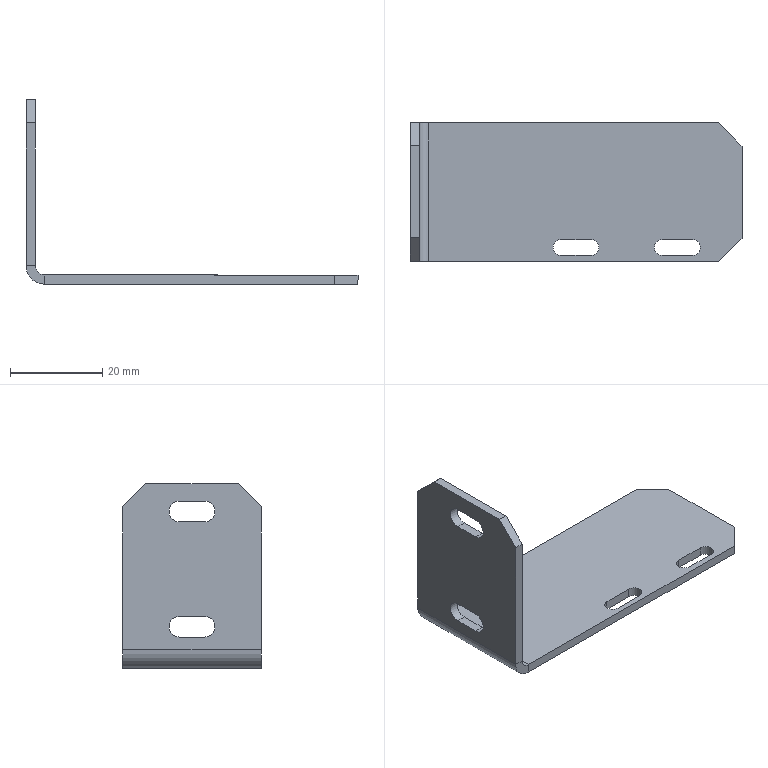Part | SolidWorks | features HoleWzd 2, Chamfer 1, EdgeFlange 1, FlatPattern 1, SMBaseFlange 1, SheetMetal 1 | 1 solid | 34 faces | box 72 x 30 x 40 mm | volume 6134 mm3 | plane 24 | cylinder 10 | commonest cylinder face diameters 3.4 x4 4.5 x4 4 x1 8 x1
STEP:
#1=CARTESIAN_POINT('',(37.3,-10.3,-20.));
#2=VERTEX_POINT('',#1);
#3=CARTESIAN_POINT('',(37.3,-13.7,-20.));
#4=VERTEX_POINT('',#3);
#5=CARTESIAN_POINT('',(37.3,-12.,-20.));
#6=DIRECTION('',(0.,0.,-1.));
#7=DIRECTION('',(0.,1.,0.));
#8=AXIS2_PLACEMENT_3D('',#5,#6,#7);
#9=CIRCLE('',#8,1.7);
#10=EDGE_CURVE('',#2,#4,#9,.T.);
#11=ORIENTED_EDGE('',*,*,#10,.F.);
#12=CARTESIAN_POINT('',(30.7,-10.3,-20.));
#13=VERTEX_POINT('',#12);
#14=CARTESIAN_POINT('',(37.3,-10.3,-20.));
#15=DIRECTION('',(-1.,0.,0.));
#16=VECTOR('',#15,1000.);
#17=LINE('',#14,#16);
#18=EDGE_CURVE('',#2,#13,#17,.T.);
#19=ORIENTED_EDGE('',*,*,#18,.T.);
#20=CARTESIAN_POINT('',(30.7,-13.7,-20.));
#21=VERTEX_POINT('',#20);
#22=CARTESIAN_POINT('',(30.7,-12.,-20.));
#23=DIRECTION('',(0.,0.,-1.));
#24=DIRECTION('',(0.,1.,0.));
#25=AXIS2_PLACEMENT_3D('',#22,#23,#24);
#26=CIRCLE('',#25,1.7);
#27=EDGE_CURVE('',#21,#13,#26,.T.);
#28=ORIENTED_EDGE('',*,*,#27,.F.);
#29=CARTESIAN_POINT('',(37.3,-13.7,-20.));
#30=DIRECTION('',(-1.,0.,0.));
#31=VECTOR('',#30,1000.);
#32=LINE('',#29,#31);
#33=EDGE_CURVE('',#4,#21,#32,.T.);
#34=ORIENTED_EDGE('',*,*,#33,.F.);
#35=EDGE_LOOP('',(#11,#19,#28,#34));
#36=FACE_BOUND('',#35,.T.);
#37=CARTESIAN_POINT('',(70.,10.,-20.));
#38=VERTEX_POINT('',#37);
#39=CARTESIAN_POINT('',(70.,-10.,-20.));
#40=VERTEX_POINT('',#39);
#41=CARTESIAN_POINT('',(70.,0.,-20.));
#42=DIRECTION('',(0.,-1.,0.));
#43=VECTOR('',#42,1000.);
#44=LINE('',#41,#43);
#45=EDGE_CURVE('',#38,#40,#44,.T.);
#46=ORIENTED_EDGE('',*,*,#45,.T.);
#47=CARTESIAN_POINT('',(65.,-15.,-20.));
#48=VERTEX_POINT('',#47);
#49=CARTESIAN_POINT('',(65.,-15.,-20.));
#50=DIRECTION('',(-0.7071,-0.7071,0.));
#51=VECTOR('',#50,1000.);
#52=LINE('',#49,#51);
#53=EDGE_CURVE('',#40,#48,#52,.T.);
#54=ORIENTED_EDGE('',*,*,#53,.T.);
#55=CARTESIAN_POINT('',(2.,-15.,-20.));
#56=VERTEX_POINT('',#55);
#57=CARTESIAN_POINT('',(0.,-15.,-20.));
#58=DIRECTION('',(-1.,0.,0.));
#59=VECTOR('',#58,1000.);
#60=LINE('',#57,#59);
#61=EDGE_CURVE('',#48,#56,#60,.T.);
#62=ORIENTED_EDGE('',*,*,#61,.T.);
#63=CARTESIAN_POINT('',(2.,15.,-20.));
#64=VERTEX_POINT('',#63);
#65=CARTESIAN_POINT('',(2.,-15.,-20.));
#66=DIRECTION('',(0.,-1.,0.));
#67=VECTOR('',#66,1000.);
#68=LINE('',#65,#67);
#69=EDGE_CURVE('',#64,#56,#68,.T.);
#70=ORIENTED_EDGE('',*,*,#69,.F.);
#71=CARTESIAN_POINT('',(65.,15.,-20.));
#72=VERTEX_POINT('',#71);
#73=CARTESIAN_POINT('',(0.,15.,-20.));
#74=DIRECTION('',(1.,0.,0.));
#75=VECTOR('',#74,1000.);
#76=LINE('',#73,#75);
#77=EDGE_CURVE('',#64,#72,#76,.T.);
#78=ORIENTED_EDGE('',*,*,#77,.T.);
#79=CARTESIAN_POINT('',(70.,10.,-20.));
#80=DIRECTION('',(0.7071,-0.7071,0.));
#81=VECTOR('',#80,1000.);
#82=LINE('',#79,#81);
#83=EDGE_CURVE('',#72,#38,#82,.T.);
#84=ORIENTED_EDGE('',*,*,#83,.T.);
#85=EDGE_LOOP('',(#46,#54,#62,#70,#78,#84));
#86=FACE_OUTER_BOUND('',#85,.T.);
#87=CARTESIAN_POINT('',(52.7,-13.7,-20.));
#88=VERTEX_POINT('',#87);
#89=CARTESIAN_POINT('',(52.7,-10.3,-20.));
#90=VERTEX_POINT('',#89);
#91=CARTESIAN_POINT('',(52.7,-12.,-20.));
#92=DIRECTION('',(0.,0.,-1.));
#93=DIRECTION('',(0.,1.,0.));
#94=AXIS2_PLACEMENT_3D('',#91,#92,#93);
#95=CIRCLE('',#94,1.7);
#96=EDGE_CURVE('',#88,#90,#95,.T.);
#97=ORIENTED_EDGE('',*,*,#96,.F.);
#98=CARTESIAN_POINT('',(59.3,-13.7,-20.));
#99=VERTEX_POINT('',#98);
#100=CARTESIAN_POINT('',(59.3,-13.7,-20.));
#101=DIRECTION('',(-1.,0.,0.));
#102=VECTOR('',#101,1000.);
#103=LINE('',#100,#102);
#104=EDGE_CURVE('',#99,#88,#103,.T.);
#105=ORIENTED_EDGE('',*,*,#104,.F.);
#106=CARTESIAN_POINT('',(59.3,-10.3,-20.));
#107=VERTEX_POINT('',#106);
#108=CARTESIAN_POINT('',(59.3,-12.,-20.));
#109=DIRECTION('',(0.,0.,-1.));
#110=DIRECTION('',(0.,1.,0.));
#111=AXIS2_PLACEMENT_3D('',#108,#109,#110);
#112=CIRCLE('',#111,1.7);
#113=EDGE_CURVE('',#107,#99,#112,.T.);
#114=ORIENTED_EDGE('',*,*,#113,.F.);
#115=CARTESIAN_POINT('',(59.3,-10.3,-20.));
#116=DIRECTION('',(-1.,0.,0.));
#117=VECTOR('',#116,1000.);
#118=LINE('',#115,#117);
#119=EDGE_CURVE('',#107,#90,#118,.T.);
#120=ORIENTED_EDGE('',*,*,#119,.T.);
#121=EDGE_LOOP('',(#97,#105,#114,#120));
#122=FACE_BOUND('',#121,.T.);
#123=CARTESIAN_POINT('',(0.,0.,-20.));
#124=DIRECTION('',(0.,0.,1.));
#125=DIRECTION('',(1.,0.,0.));
#126=AXIS2_PLACEMENT_3D('',#123,#124,#125);
#127=PLANE('',#126);
#128=ADVANCED_FACE('',(#36,#86,#122),#127,.F.);
#129=CARTESIAN_POINT('',(-2.,15.,-16.));
#130=VERTEX_POINT('',#129);
#131=CARTESIAN_POINT('',(-2.,15.,15.));
#132=VERTEX_POINT('',#131);
#133=CARTESIAN_POINT('',(-2.,15.,20.));
#134=DIRECTION('',(0.,0.,1.));
#135=VECTOR('',#134,1000.);
#136=LINE('',#133,#135);
#137=EDGE_CURVE('',#130,#132,#136,.T.);
#138=ORIENTED_EDGE('',*,*,#137,.T.);
#139=CARTESIAN_POINT('',(0.,15.,15.));
#140=VERTEX_POINT('',#139);
#141=CARTESIAN_POINT('',(-2.,15.,15.));
#142=DIRECTION('',(1.,0.,0.));
#143=VECTOR('',#142,1000.);
#144=LINE('',#141,#143);
#145=EDGE_CURVE('',#132,#140,#144,.T.);
#146=ORIENTED_EDGE('',*,*,#145,.T.);
#147=CARTESIAN_POINT('',(0.,15.,-16.));
#148=VERTEX_POINT('',#147);
#149=CARTESIAN_POINT('',(0.,15.,20.));
#150=DIRECTION('',(0.,0.,1.));
#151=VECTOR('',#150,1000.);
#152=LINE('',#149,#151);
#153=EDGE_CURVE('',#148,#140,#152,.T.);
#154=ORIENTED_EDGE('',*,*,#153,.F.);
#155=CARTESIAN_POINT('',(0.,15.,-16.));
#156=DIRECTION('',(-1.,0.,0.));
#157=VECTOR('',#156,1000.);
#158=LINE('',#155,#157);
#159=EDGE_CURVE('',#148,#130,#158,.T.);
#160=ORIENTED_EDGE('',*,*,#159,.T.);
#161=EDGE_LOOP('',(#138,#146,#154,#160));
#162=FACE_OUTER_BOUND('',#161,.T.);
#163=CARTESIAN_POINT('',(-2.,15.,20.));
#164=DIRECTION('',(0.,1.,0.));
#165=DIRECTION('',(0.,0.,1.));
#166=AXIS2_PLACEMENT_3D('',#163,#164,#165);
#167=PLANE('',#166);
#168=ADVANCED_FACE('',(#162),#167,.T.);
#169=CARTESIAN_POINT('',(-2.,2.75,11.75));
#170=VERTEX_POINT('',#169);
#171=CARTESIAN_POINT('',(-2.,2.75,16.25));
#172=VERTEX_POINT('',#171);
#173=CARTESIAN_POINT('',(-2.,2.75,14.));
#174=DIRECTION('',(1.,0.,0.));
#175=DIRECTION('',(0.,0.,-1.));
#176=AXIS2_PLACEMENT_3D('',#173,#174,#175);
#177=CIRCLE('',#176,2.25);
#178=EDGE_CURVE('',#170,#172,#177,.T.);
#179=ORIENTED_EDGE('',*,*,#178,.T.);
#180=CARTESIAN_POINT('',(-2.,-2.75,16.25));
#181=VERTEX_POINT('',#180);
#182=CARTESIAN_POINT('',(-2.,2.75,16.25));
#183=DIRECTION('',(0.,-1.,0.));
#184=VECTOR('',#183,1000.);
#185=LINE('',#182,#184);
#186=EDGE_CURVE('',#172,#181,#185,.T.);
#187=ORIENTED_EDGE('',*,*,#186,.T.);
#188=CARTESIAN_POINT('',(-2.,-2.75,11.75));
#189=VERTEX_POINT('',#188);
#190=CARTESIAN_POINT('',(-2.,-2.75,14.));
#191=DIRECTION('',(1.,0.,0.));
#192=DIRECTION('',(0.,0.,-1.));
#193=AXIS2_PLACEMENT_3D('',#190,#191,#192);
#194=CIRCLE('',#193,2.25);
#195=EDGE_CURVE('',#181,#189,#194,.T.);
#196=ORIENTED_EDGE('',*,*,#195,.T.);
#197=CARTESIAN_POINT('',(-2.,2.75,11.75));
#198=DIRECTION('',(0.,-1.,0.));
#199=VECTOR('',#198,1000.);
#200=LINE('',#197,#199);
#201=EDGE_CURVE('',#170,#189,#200,.T.);
#202=ORIENTED_EDGE('',*,*,#201,.F.);
#203=EDGE_LOOP('',(#179,#187,#196,#202));
#204=FACE_BOUND('',#203,.T.);
#205=CARTESIAN_POINT('',(-2.,2.75,-13.25));
#206=VERTEX_POINT('',#205);
#207=CARTESIAN_POINT('',(-2.,2.75,-8.75));
#208=VERTEX_POINT('',#207);
#209=CARTESIAN_POINT('',(-2.,2.75,-11.));
#210=DIRECTION('',(1.,0.,0.));
#211=DIRECTION('',(0.,0.,-1.));
#212=AXIS2_PLACEMENT_3D('',#209,#210,#211);
#213=CIRCLE('',#212,2.25);
#214=EDGE_CURVE('',#206,#208,#213,.T.);
#215=ORIENTED_EDGE('',*,*,#214,.T.);
#216=CARTESIAN_POINT('',(-2.,-2.75,-8.75));
#217=VERTEX_POINT('',#216);
#218=CARTESIAN_POINT('',(-2.,2.75,-8.75));
#219=DIRECTION('',(0.,-1.,0.));
#220=VECTOR('',#219,1000.);
#221=LINE('',#218,#220);
#222=EDGE_CURVE('',#208,#217,#221,.T.);
#223=ORIENTED_EDGE('',*,*,#222,.T.);
#224=CARTESIAN_POINT('',(-2.,-2.75,-13.25));
#225=VERTEX_POINT('',#224);
#226=CARTESIAN_POINT('',(-2.,-2.75,-11.));
#227=DIRECTION('',(1.,0.,0.));
#228=DIRECTION('',(0.,0.,-1.));
#229=AXIS2_PLACEMENT_3D('',#226,#227,#228);
#230=CIRCLE('',#229,2.25);
#231=EDGE_CURVE('',#217,#225,#230,.T.);
#232=ORIENTED_EDGE('',*,*,#231,.T.);
#233=CARTESIAN_POINT('',(-2.,2.75,-13.25));
#234=DIRECTION('',(0.,-1.,0.));
#235=VECTOR('',#234,1000.);
#236=LINE('',#233,#235);
#237=EDGE_CURVE('',#206,#225,#236,.T.);
#238=ORIENTED_EDGE('',*,*,#237,.F.);
#239=EDGE_LOOP('',(#215,#223,#232,#238));
#240=FACE_BOUND('',#239,.T.);
#241=CARTESIAN_POINT('',(-2.,-15.,15.));
#242=VERTEX_POINT('',#241);
#243=CARTESIAN_POINT('',(-2.,-15.,-16.));
#244=VERTEX_POINT('',#243);
#245=CARTESIAN_POINT('',(-2.,-15.,20.));
#246=DIRECTION('',(0.,0.,-1.));
#247=VECTOR('',#246,1000.);
#248=LINE('',#245,#247);
#249=EDGE_CURVE('',#242,#244,#248,.T.);
#250=ORIENTED_EDGE('',*,*,#249,.F.);
#251=CARTESIAN_POINT('',(-2.,-10.,20.));
#252=VERTEX_POINT('',#251);
#253=CARTESIAN_POINT('',(-2.,-10.,20.));
#254=DIRECTION('',(0.,0.7071,0.7071));
#255=VECTOR('',#254,1000.);
#256=LINE('',#253,#255);
#257=EDGE_CURVE('',#242,#252,#256,.T.);
#258=ORIENTED_EDGE('',*,*,#257,.T.);
#259=CARTESIAN_POINT('',(-2.,10.,20.));
#260=VERTEX_POINT('',#259);
#261=CARTESIAN_POINT('',(-2.,15.,20.));
#262=DIRECTION('',(0.,-1.,0.));
#263=VECTOR('',#262,1000.);
#264=LINE('',#261,#263);
#265=EDGE_CURVE('',#260,#252,#264,.T.);
#266=ORIENTED_EDGE('',*,*,#265,.F.);
#267=CARTESIAN_POINT('',(-2.,15.,15.));
#268=DIRECTION('',(0.,0.7071,-0.7071));
#269=VECTOR('',#268,1000.);
#270=LINE('',#267,#269);
#271=EDGE_CURVE('',#260,#132,#270,.T.);
#272=ORIENTED_EDGE('',*,*,#271,.T.);
#273=ORIENTED_EDGE('',*,*,#137,.F.);
#274=CARTESIAN_POINT('',(-2.,15.,-16.));
#275=DIRECTION('',(0.,-1.,0.));
#276=VECTOR('',#275,1000.);
#277=LINE('',#274,#276);
#278=EDGE_CURVE('',#130,#244,#277,.T.);
#279=ORIENTED_EDGE('',*,*,#278,.T.);
#280=EDGE_LOOP('',(#250,#258,#266,#272,#273,#279));
#281=FACE_OUTER_BOUND('',#280,.T.);
#282=CARTESIAN_POINT('',(-2.,0.,0.));
#283=DIRECTION('',(1.,0.,0.));
#284=DIRECTION('',(0.,0.,-1.));
#285=AXIS2_PLACEMENT_3D('',#282,#283,#284);
#286=PLANE('',#285);
#287=ADVANCED_FACE('',(#204,#240,#281),#286,.F.);
#288=CARTESIAN_POINT('',(0.,2.75,11.75));
#289=VERTEX_POINT('',#288);
#290=CARTESIAN_POINT('',(0.,2.75,16.25));
#291=VERTEX_POINT('',#290);
#292=CARTESIAN_POINT('',(0.,2.75,14.));
#293=DIRECTION('',(1.,0.,0.));
#294=DIRECTION('',(0.,0.,-1.));
#295=AXIS2_PLACEMENT_3D('',#292,#293,#294);
#296=CIRCLE('',#295,2.25);
#297=EDGE_CURVE('',#289,#291,#296,.T.);
#298=ORIENTED_EDGE('',*,*,#297,.F.);
#299=CARTESIAN_POINT('',(0.,-2.75,11.75));
#300=VERTEX_POINT('',#299);
#301=CARTESIAN_POINT('',(0.,2.75,11.75));
#302=DIRECTION('',(0.,-1.,0.));
#303=VECTOR('',#302,1000.);
#304=LINE('',#301,#303);
#305=EDGE_CURVE('',#289,#300,#304,.T.);
#306=ORIENTED_EDGE('',*,*,#305,.T.);
#307=CARTESIAN_POINT('',(0.,-2.75,16.25));
#308=VERTEX_POINT('',#307);
#309=CARTESIAN_POINT('',(0.,-2.75,14.));
#310=DIRECTION('',(1.,0.,0.));
#311=DIRECTION('',(0.,0.,-1.));
#312=AXIS2_PLACEMENT_3D('',#309,#310,#311);
#313=CIRCLE('',#312,2.25);
#314=EDGE_CURVE('',#308,#300,#313,.T.);
#315=ORIENTED_EDGE('',*,*,#314,.F.);
#316=CARTESIAN_POINT('',(0.,2.75,16.25));
#317=DIRECTION('',(0.,-1.,0.));
#318=VECTOR('',#317,1000.);
#319=LINE('',#316,#318);
#320=EDGE_CURVE('',#291,#308,#319,.T.);
#321=ORIENTED_EDGE('',*,*,#320,.F.);
#322=EDGE_LOOP('',(#298,#306,#315,#321));
#323=FACE_BOUND('',#322,.T.);
#324=CARTESIAN_POINT('',(0.,2.75,-13.25));
#325=VERTEX_POINT('',#324);
#326=CARTESIAN_POINT('',(0.,-2.75,-13.25));
#327=VERTEX_POINT('',#326);
#328=CARTESIAN_POINT('',(0.,2.75,-13.25));
#329=DIRECTION('',(0.,-1.,0.));
#330=VECTOR('',#329,1000.);
#331=LINE('',#328,#330);
#332=EDGE_CURVE('',#325,#327,#331,.T.);
#333=ORIENTED_EDGE('',*,*,#332,.T.);
#334=CARTESIAN_POINT('',(0.,-2.75,-8.75));
#335=VERTEX_POINT('',#334);
#336=CARTESIAN_POINT('',(0.,-2.75,-11.));
#337=DIRECTION('',(1.,0.,0.));
#338=DIRECTION('',(0.,0.,-1.));
#339=AXIS2_PLACEMENT_3D('',#336,#337,#338);
#340=CIRCLE('',#339,2.25);
#341=EDGE_CURVE('',#335,#327,#340,.T.);
#342=ORIENTED_EDGE('',*,*,#341,.F.);
#343=CARTESIAN_POINT('',(0.,2.75,-8.75));
#344=VERTEX_POINT('',#343);
#345=CARTESIAN_POINT('',(0.,2.75,-8.75));
#346=DIRECTION('',(0.,-1.,0.));
#347=VECTOR('',#346,1000.);
#348=LINE('',#345,#347);
#349=EDGE_CURVE('',#344,#335,#348,.T.);
#350=ORIENTED_EDGE('',*,*,#349,.F.);
#351=CARTESIAN_POINT('',(0.,2.75,-11.));
#352=DIRECTION('',(1.,0.,0.));
#353=DIRECTION('',(0.,0.,-1.));
#354=AXIS2_PLACEMENT_3D('',#351,#352,#353);
#355=CIRCLE('',#354,2.25);
#356=EDGE_CURVE('',#325,#344,#355,.T.);
#357=ORIENTED_EDGE('',*,*,#356,.F.);
#358=EDGE_LOOP('',(#333,#342,#350,#357));
#359=FACE_BOUND('',#358,.T.);
#360=CARTESIAN_POINT('',(0.,10.,20.));
#361=VERTEX_POINT('',#360);
#362=CARTESIAN_POINT('',(0.,-10.,20.));
#363=VERTEX_POINT('',#362);
#364=CARTESIAN_POINT('',(0.,15.,20.));
#365=DIRECTION('',(0.,-1.,0.));
#366=VECTOR('',#365,1000.);
#367=LINE('',#364,#366);
#368=EDGE_CURVE('',#361,#363,#367,.T.);
#369=ORIENTED_EDGE('',*,*,#368,.T.);
#370=CARTESIAN_POINT('',(0.,-15.,15.));
#371=VERTEX_POINT('',#370);
#372=CARTESIAN_POINT('',(0.,-15.,15.));
#373=DIRECTION('',(0.,-0.7071,-0.7071));
#374=VECTOR('',#373,1000.);
#375=LINE('',#372,#374);
#376=EDGE_CURVE('',#363,#371,#375,.T.);
#377=ORIENTED_EDGE('',*,*,#376,.T.);
#378=CARTESIAN_POINT('',(0.,-15.,-16.));
#379=VERTEX_POINT('',#378);
#380=CARTESIAN_POINT('',(0.,-15.,20.));
#381=DIRECTION('',(0.,0.,-1.));
#382=VECTOR('',#381,1000.);
#383=LINE('',#380,#382);
#384=EDGE_CURVE('',#371,#379,#383,.T.);
#385=ORIENTED_EDGE('',*,*,#384,.T.);
#386=CARTESIAN_POINT('',(0.,15.,-16.));
#387=DIRECTION('',(0.,-1.,0.));
#388=VECTOR('',#387,1000.);
#389=LINE('',#386,#388);
#390=EDGE_CURVE('',#148,#379,#389,.T.);
#391=ORIENTED_EDGE('',*,*,#390,.F.);
#392=ORIENTED_EDGE('',*,*,#153,.T.);
#393=CARTESIAN_POINT('',(0.,15.,15.));
#394=DIRECTION('',(0.,-0.7071,0.7071));
#395=VECTOR('',#394,1000.);
#396=LINE('',#393,#395);
#397=EDGE_CURVE('',#140,#361,#396,.T.);
#398=ORIENTED_EDGE('',*,*,#397,.T.);
#399=EDGE_LOOP('',(#369,#377,#385,#391,#392,#398));
#400=FACE_OUTER_BOUND('',#399,.T.);
#401=CARTESIAN_POINT('',(0.,0.,0.));
#402=DIRECTION('',(1.,0.,0.));
#403=DIRECTION('',(0.,0.,-1.));
#404=AXIS2_PLACEMENT_3D('',#401,#402,#403);
#405=PLANE('',#404);
#406=ADVANCED_FACE('',(#323,#359,#400),#405,.T.);
#407=ORIENTED_EDGE('',*,*,#384,.F.);
#408=CARTESIAN_POINT('',(-2.,-15.,15.));
#409=DIRECTION('',(-1.,0.,0.));
#410=VECTOR('',#409,1000.);
#411=LINE('',#408,#410);
#412=EDGE_CURVE('',#371,#242,#411,.T.);
#413=ORIENTED_EDGE('',*,*,#412,.T.);
#414=ORIENTED_EDGE('',*,*,#249,.T.);
#415=CARTESIAN_POINT('',(0.,-15.,-16.));
#416=DIRECTION('',(-1.,0.,0.));
#417=VECTOR('',#416,1000.);
#418=LINE('',#415,#417);
#419=EDGE_CURVE('',#379,#244,#418,.T.);
#420=ORIENTED_EDGE('',*,*,#419,.F.);
#421=EDGE_LOOP('',(#407,#413,#414,#420));
#422=FACE_OUTER_BOUND('',#421,.T.);
#423=CARTESIAN_POINT('',(-2.,-15.,20.));
#424=DIRECTION('',(0.,-1.,0.));
#425=DIRECTION('',(0.,0.,-1.));
#426=AXIS2_PLACEMENT_3D('',#423,#424,#425);
#427=PLANE('',#426);
#428=ADVANCED_FACE('',(#422),#427,.T.);
#429=ORIENTED_EDGE('',*,*,#265,.T.);
#430=CARTESIAN_POINT('',(-2.,-10.,20.));
#431=DIRECTION('',(1.,0.,0.));
#432=VECTOR('',#431,1000.);
#433=LINE('',#430,#432);
#434=EDGE_CURVE('',#252,#363,#433,.T.);
#435=ORIENTED_EDGE('',*,*,#434,.T.);
#436=ORIENTED_EDGE('',*,*,#368,.F.);
#437=CARTESIAN_POINT('',(-2.,10.,20.));
#438=DIRECTION('',(-1.,0.,0.));
#439=VECTOR('',#438,1000.);
#440=LINE('',#437,#439);
#441=EDGE_CURVE('',#361,#260,#440,.T.);
#442=ORIENTED_EDGE('',*,*,#441,.T.);
#443=EDGE_LOOP('',(#429,#435,#436,#442));
#444=FACE_OUTER_BOUND('',#443,.T.);
#445=CARTESIAN_POINT('',(-2.,15.,20.));
#446=DIRECTION('',(0.,0.,1.));
#447=DIRECTION('',(0.,-1.,0.));
#448=AXIS2_PLACEMENT_3D('',#445,#446,#447);
#449=PLANE('',#448);
#450=ADVANCED_FACE('',(#444),#449,.T.);
#451=CARTESIAN_POINT('',(2.,-15.,-18.));
#452=VERTEX_POINT('',#451);
#453=CARTESIAN_POINT('',(2.,-15.,-20.));
#454=DIRECTION('',(0.,0.,-1.));
#455=VECTOR('',#454,1000.);
#456=LINE('',#453,#455);
#457=EDGE_CURVE('',#452,#56,#456,.T.);
#458=ORIENTED_EDGE('',*,*,#457,.F.);
#459=CARTESIAN_POINT('',(2.,-15.,-16.));
#460=DIRECTION('',(0.,-1.,0.));
#461=DIRECTION('',(0.,0.,1.));
#462=AXIS2_PLACEMENT_3D('',#459,#460,#461);
#463=CIRCLE('',#462,2.);
#464=EDGE_CURVE('',#379,#452,#463,.T.);
#465=ORIENTED_EDGE('',*,*,#464,.F.);
#466=ORIENTED_EDGE('',*,*,#419,.T.);
#467=CARTESIAN_POINT('',(2.,-15.,-16.));
#468=DIRECTION('',(0.,-1.,0.));
#469=DIRECTION('',(0.,0.,1.));
#470=AXIS2_PLACEMENT_3D('',#467,#468,#469);
#471=CIRCLE('',#470,4.);
#472=EDGE_CURVE('',#244,#56,#471,.T.);
#473=ORIENTED_EDGE('',*,*,#472,.T.);
#474=EDGE_LOOP('',(#458,#465,#466,#473));
#475=FACE_OUTER_BOUND('',#474,.T.);
#476=CARTESIAN_POINT('',(2.,-15.,-16.));
#477=DIRECTION('',(0.,-1.,0.));
#478=DIRECTION('',(0.,0.,-1.));
#479=AXIS2_PLACEMENT_3D('',#476,#477,#478);
#480=PLANE('',#479);
#481=ADVANCED_FACE('',(#475),#480,.T.);
#482=CARTESIAN_POINT('',(2.,15.,-18.));
#483=VERTEX_POINT('',#482);
#484=CARTESIAN_POINT('',(2.,15.,-16.));
#485=DIRECTION('',(0.,1.,0.));
#486=DIRECTION('',(0.,0.,1.));
#487=AXIS2_PLACEMENT_3D('',#484,#485,#486);
#488=CIRCLE('',#487,2.);
#489=EDGE_CURVE('',#483,#148,#488,.T.);
#490=ORIENTED_EDGE('',*,*,#489,.F.);
#491=CARTESIAN_POINT('',(2.,15.,-18.));
#492=DIRECTION('',(0.,0.,-1.));
#493=VECTOR('',#492,1000.);
#494=LINE('',#491,#493);
#495=EDGE_CURVE('',#483,#64,#494,.T.);
#496=ORIENTED_EDGE('',*,*,#495,.T.);
#497=CARTESIAN_POINT('',(2.,15.,-16.));
#498=DIRECTION('',(0.,1.,0.));
#499=DIRECTION('',(0.,0.,1.));
#500=AXIS2_PLACEMENT_3D('',#497,#498,#499);
#501=CIRCLE('',#500,4.);
#502=EDGE_CURVE('',#64,#130,#501,.T.);
#503=ORIENTED_EDGE('',*,*,#502,.T.);
#504=ORIENTED_EDGE('',*,*,#159,.F.);
#505=EDGE_LOOP('',(#490,#496,#503,#504));
#506=FACE_OUTER_BOUND('',#505,.T.);
#507=CARTESIAN_POINT('',(2.,15.,-16.));
#508=DIRECTION('',(0.,-1.,0.));
#509=DIRECTION('',(0.,0.,-1.));
#510=AXIS2_PLACEMENT_3D('',#507,#508,#509);
#511=PLANE('',#510);
#512=ADVANCED_FACE('',(#506),#511,.F.);
#513=ORIENTED_EDGE('',*,*,#278,.F.);
#514=ORIENTED_EDGE('',*,*,#502,.F.);
#515=ORIENTED_EDGE('',*,*,#69,.T.);
#516=ORIENTED_EDGE('',*,*,#472,.F.);
#517=EDGE_LOOP('',(#513,#514,#515,#516));
#518=FACE_OUTER_BOUND('',#517,.T.);
#519=CARTESIAN_POINT('',(2.,15.,-16.));
#520=DIRECTION('',(0.,1.,0.));
#521=DIRECTION('',(0.,0.,-1.));
#522=AXIS2_PLACEMENT_3D('',#519,#520,#521);
#523=CYLINDRICAL_SURFACE('',#522,4.);
#524=ADVANCED_FACE('',(#518),#523,.T.);
#525=ORIENTED_EDGE('',*,*,#390,.T.);
#526=ORIENTED_EDGE('',*,*,#464,.T.);
#527=CARTESIAN_POINT('',(2.,-15.,-18.));
#528=DIRECTION('',(0.,1.,0.));
#529=VECTOR('',#528,1000.);
#530=LINE('',#527,#529);
#531=EDGE_CURVE('',#452,#483,#530,.T.);
#532=ORIENTED_EDGE('',*,*,#531,.T.);
#533=ORIENTED_EDGE('',*,*,#489,.T.);
#534=EDGE_LOOP('',(#525,#526,#532,#533));
#535=FACE_OUTER_BOUND('',#534,.T.);
#536=CARTESIAN_POINT('',(2.,15.,-16.));
#537=DIRECTION('',(0.,1.,0.));
#538=DIRECTION('',(0.,0.,-1.));
#539=AXIS2_PLACEMENT_3D('',#536,#537,#538);
#540=CYLINDRICAL_SURFACE('',#539,2.);
#541=ADVANCED_FACE('',(#535),#540,.F.);
#542=ORIENTED_EDGE('',*,*,#61,.F.);
#543=CARTESIAN_POINT('',(65.,-15.,-18.));
#544=VERTEX_POINT('',#543);
#545=CARTESIAN_POINT('',(65.,-15.,-20.));
#546=DIRECTION('',(0.,0.,1.));
#547=VECTOR('',#546,1000.);
#548=LINE('',#545,#547);
#549=EDGE_CURVE('',#48,#544,#548,.T.);
#550=ORIENTED_EDGE('',*,*,#549,.T.);
#551=CARTESIAN_POINT('',(0.,-15.,-18.));
#552=DIRECTION('',(-1.,0.,0.));
#553=VECTOR('',#552,1000.);
#554=LINE('',#551,#553);
#555=EDGE_CURVE('',#544,#452,#554,.T.);
#556=ORIENTED_EDGE('',*,*,#555,.T.);
#557=ORIENTED_EDGE('',*,*,#457,.T.);
#558=EDGE_LOOP('',(#542,#550,#556,#557));
#559=FACE_OUTER_BOUND('',#558,.T.);
#560=CARTESIAN_POINT('',(0.,-15.,-20.));
#561=DIRECTION('',(0.,1.,0.));
#562=DIRECTION('',(0.,0.,1.));
#563=AXIS2_PLACEMENT_3D('',#560,#561,#562);
#564=PLANE('',#563);
#565=ADVANCED_FACE('',(#559),#564,.F.);
#566=CARTESIAN_POINT('',(65.,15.,-18.));
#567=VERTEX_POINT('',#566);
#568=CARTESIAN_POINT('',(70.,15.,-18.));
#569=DIRECTION('',(1.,0.,0.));
#570=VECTOR('',#569,1000.);
#571=LINE('',#568,#570);
#572=EDGE_CURVE('',#483,#567,#571,.T.);
#573=ORIENTED_EDGE('',*,*,#572,.T.);
#574=CARTESIAN_POINT('',(65.,15.,-20.));
#575=DIRECTION('',(0.,0.,-1.));
#576=VECTOR('',#575,1000.);
#577=LINE('',#574,#576);
#578=EDGE_CURVE('',#567,#72,#577,.T.);
#579=ORIENTED_EDGE('',*,*,#578,.T.);
#580=ORIENTED_EDGE('',*,*,#77,.F.);
#581=ORIENTED_EDGE('',*,*,#495,.F.);
#582=EDGE_LOOP('',(#573,#579,#580,#581));
#583=FACE_OUTER_BOUND('',#582,.T.);
#584=CARTESIAN_POINT('',(70.,15.,-20.));
#585=DIRECTION('',(0.,-1.,0.));
#586=DIRECTION('',(0.,0.,-1.));
#587=AXIS2_PLACEMENT_3D('',#584,#585,#586);
#588=PLANE('',#587);
#589=ADVANCED_FACE('',(#583),#588,.F.);
#590=CARTESIAN_POINT('',(59.3,-10.3,-18.));
#591=VERTEX_POINT('',#590);
#592=CARTESIAN_POINT('',(52.7,-10.3,-18.));
#593=VERTEX_POINT('',#592);
#594=CARTESIAN_POINT('',(0.,-10.3,-18.));
#595=DIRECTION('',(-1.,0.,0.));
#596=VECTOR('',#595,1000.);
#597=LINE('',#594,#596);
#598=EDGE_CURVE('',#591,#593,#597,.T.);
#599=ORIENTED_EDGE('',*,*,#598,.F.);
#600=CARTESIAN_POINT('',(59.3,-13.7,-18.));
#601=VERTEX_POINT('',#600);
#602=CARTESIAN_POINT('',(59.3,-12.,-18.));
#603=DIRECTION('',(0.,0.,1.));
#604=DIRECTION('',(1.,0.,0.));
#605=AXIS2_PLACEMENT_3D('',#602,#603,#604);
#606=CIRCLE('',#605,1.7);
#607=EDGE_CURVE('',#601,#591,#606,.T.);
#608=ORIENTED_EDGE('',*,*,#607,.F.);
#609=CARTESIAN_POINT('',(52.7,-13.7,-18.));
#610=VERTEX_POINT('',#609);
#611=CARTESIAN_POINT('',(0.,-13.7,-18.));
#612=DIRECTION('',(1.,0.,0.));
#613=VECTOR('',#612,1000.);
#614=LINE('',#611,#613);
#615=EDGE_CURVE('',#610,#601,#614,.T.);
#616=ORIENTED_EDGE('',*,*,#615,.F.);
#617=CARTESIAN_POINT('',(52.7,-12.,-18.));
#618=DIRECTION('',(0.,0.,1.));
#619=DIRECTION('',(1.,0.,0.));
#620=AXIS2_PLACEMENT_3D('',#617,#618,#619);
#621=CIRCLE('',#620,1.7);
#622=EDGE_CURVE('',#593,#610,#621,.T.);
#623=ORIENTED_EDGE('',*,*,#622,.F.);
#624=EDGE_LOOP('',(#599,#608,#616,#623));
#625=FACE_BOUND('',#624,.T.);
#626=CARTESIAN_POINT('',(30.7,-10.3,-18.));
#627=VERTEX_POINT('',#626);
#628=CARTESIAN_POINT('',(30.7,-13.7,-18.));
#629=VERTEX_POINT('',#628);
#630=CARTESIAN_POINT('',(30.7,-12.,-18.));
#631=DIRECTION('',(0.,0.,1.));
#632=DIRECTION('',(1.,0.,0.));
#633=AXIS2_PLACEMENT_3D('',#630,#631,#632);
#634=CIRCLE('',#633,1.7);
#635=EDGE_CURVE('',#627,#629,#634,.T.);
#636=ORIENTED_EDGE('',*,*,#635,.F.);
#637=CARTESIAN_POINT('',(37.3,-10.3,-18.));
#638=VERTEX_POINT('',#637);
#639=CARTESIAN_POINT('',(0.,-10.3,-18.));
#640=DIRECTION('',(-1.,0.,0.));
#641=VECTOR('',#640,1000.);
#642=LINE('',#639,#641);
#643=EDGE_CURVE('',#638,#627,#642,.T.);
#644=ORIENTED_EDGE('',*,*,#643,.F.);
#645=CARTESIAN_POINT('',(37.3,-13.7,-18.));
#646=VERTEX_POINT('',#645);
#647=CARTESIAN_POINT('',(37.3,-12.,-18.));
#648=DIRECTION('',(0.,0.,1.));
#649=DIRECTION('',(1.,0.,0.));
#650=AXIS2_PLACEMENT_3D('',#647,#648,#649);
#651=CIRCLE('',#650,1.7);
#652=EDGE_CURVE('',#646,#638,#651,.T.);
#653=ORIENTED_EDGE('',*,*,#652,.F.);
#654=CARTESIAN_POINT('',(0.,-13.7,-18.));
#655=DIRECTION('',(1.,0.,0.));
#656=VECTOR('',#655,1000.);
#657=LINE('',#654,#656);
#658=EDGE_CURVE('',#629,#646,#657,.T.);
#659=ORIENTED_EDGE('',*,*,#658,.F.);
#660=EDGE_LOOP('',(#636,#644,#653,#659));
#661=FACE_BOUND('',#660,.T.);
#662=ORIENTED_EDGE('',*,*,#555,.F.);
#663=CARTESIAN_POINT('',(70.,-10.,-18.));
#664=VERTEX_POINT('',#663);
#665=CARTESIAN_POINT('',(40.,-40.,-18.));
#666=DIRECTION('',(0.7071,0.7071,0.));
#667=VECTOR('',#666,1000.);
#668=LINE('',#665,#667);
#669=EDGE_CURVE('',#544,#664,#668,.T.);
#670=ORIENTED_EDGE('',*,*,#669,.T.);
#671=CARTESIAN_POINT('',(70.,10.,-18.));
#672=VERTEX_POINT('',#671);
#673=CARTESIAN_POINT('',(70.,-15.,-18.));
#674=DIRECTION('',(0.,-1.,0.));
#675=VECTOR('',#674,1000.);
#676=LINE('',#673,#675);
#677=EDGE_CURVE('',#672,#664,#676,.T.);
#678=ORIENTED_EDGE('',*,*,#677,.F.);
#679=CARTESIAN_POINT('',(40.,40.,-18.));
#680=DIRECTION('',(-0.7071,0.7071,0.));
#681=VECTOR('',#680,1000.);
#682=LINE('',#679,#681);
#683=EDGE_CURVE('',#672,#567,#682,.T.);
#684=ORIENTED_EDGE('',*,*,#683,.T.);
#685=ORIENTED_EDGE('',*,*,#572,.F.);
#686=ORIENTED_EDGE('',*,*,#531,.F.);
#687=EDGE_LOOP('',(#662,#670,#678,#684,#685,#686));
#688=FACE_OUTER_BOUND('',#687,.T.);
#689=CARTESIAN_POINT('',(0.,0.,-18.));
#690=DIRECTION('',(0.,0.,1.));
#691=DIRECTION('',(1.,0.,0.));
#692=AXIS2_PLACEMENT_3D('',#689,#690,#691);
#693=PLANE('',#692);
#694=ADVANCED_FACE('',(#625,#661,#688),#693,.T.);
#695=ORIENTED_EDGE('',*,*,#677,.T.);
#696=CARTESIAN_POINT('',(70.,-10.,-20.));
#697=DIRECTION('',(0.,0.,-1.));
#698=VECTOR('',#697,1000.);
#699=LINE('',#696,#698);
#700=EDGE_CURVE('',#664,#40,#699,.T.);
#701=ORIENTED_EDGE('',*,*,#700,.T.);
#702=ORIENTED_EDGE('',*,*,#45,.F.);
#703=CARTESIAN_POINT('',(70.,10.,-20.));
#704=DIRECTION('',(0.,0.,1.));
#705=VECTOR('',#704,1000.);
#706=LINE('',#703,#705);
#707=EDGE_CURVE('',#38,#672,#706,.T.);
#708=ORIENTED_EDGE('',*,*,#707,.T.);
#709=EDGE_LOOP('',(#695,#701,#702,#708));
#710=FACE_OUTER_BOUND('',#709,.T.);
#711=CARTESIAN_POINT('',(70.,-15.,-20.));
#712=DIRECTION('',(-1.,0.,0.));
#713=DIRECTION('',(0.,0.,1.));
#714=AXIS2_PLACEMENT_3D('',#711,#712,#713);
#715=PLANE('',#714);
#716=ADVANCED_FACE('',(#710),#715,.F.);
#717=ORIENTED_EDGE('',*,*,#257,.F.);
#718=ORIENTED_EDGE('',*,*,#412,.F.);
#719=ORIENTED_EDGE('',*,*,#376,.F.);
#720=ORIENTED_EDGE('',*,*,#434,.F.);
#721=EDGE_LOOP('',(#717,#718,#719,#720));
#722=FACE_OUTER_BOUND('',#721,.T.);
#723=CARTESIAN_POINT('',(-2.,-10.,20.));
#724=DIRECTION('',(0.,0.7071,-0.7071));
#725=DIRECTION('',(1.,0.,0.));
#726=AXIS2_PLACEMENT_3D('',#723,#724,#725);
#727=PLANE('',#726);
#728=ADVANCED_FACE('',(#722),#727,.F.);
#729=ORIENTED_EDGE('',*,*,#271,.F.);
#730=ORIENTED_EDGE('',*,*,#441,.F.);
#731=ORIENTED_EDGE('',*,*,#397,.F.);
#732=ORIENTED_EDGE('',*,*,#145,.F.);
#733=EDGE_LOOP('',(#729,#730,#731,#732));
#734=FACE_OUTER_BOUND('',#733,.T.);
#735=CARTESIAN_POINT('',(-2.,15.,15.));
#736=DIRECTION('',(0.,-0.7071,-0.7071));
#737=DIRECTION('',(1.,0.,0.));
#738=AXIS2_PLACEMENT_3D('',#735,#736,#737);
#739=PLANE('',#738);
#740=ADVANCED_FACE('',(#734),#739,.F.);
#741=ORIENTED_EDGE('',*,*,#53,.F.);
#742=ORIENTED_EDGE('',*,*,#700,.F.);
#743=ORIENTED_EDGE('',*,*,#669,.F.);
#744=ORIENTED_EDGE('',*,*,#549,.F.);
#745=EDGE_LOOP('',(#741,#742,#743,#744));
#746=FACE_OUTER_BOUND('',#745,.T.);
#747=CARTESIAN_POINT('',(65.,-15.,-20.));
#748=DIRECTION('',(-0.7071,0.7071,0.));
#749=DIRECTION('',(0.,0.,1.));
#750=AXIS2_PLACEMENT_3D('',#747,#748,#749);
#751=PLANE('',#750);
#752=ADVANCED_FACE('',(#746),#751,.F.);
#753=ORIENTED_EDGE('',*,*,#83,.F.);
#754=ORIENTED_EDGE('',*,*,#578,.F.);
#755=ORIENTED_EDGE('',*,*,#683,.F.);
#756=ORIENTED_EDGE('',*,*,#707,.F.);
#757=EDGE_LOOP('',(#753,#754,#755,#756));
#758=FACE_OUTER_BOUND('',#757,.T.);
#759=CARTESIAN_POINT('',(70.,10.,-20.));
#760=DIRECTION('',(-0.7071,-0.7071,0.));
#761=DIRECTION('',(0.,0.,1.));
#762=AXIS2_PLACEMENT_3D('',#759,#760,#761);
#763=PLANE('',#762);
#764=ADVANCED_FACE('',(#758),#763,.F.);
#765=ORIENTED_EDGE('',*,*,#341,.T.);
#766=CARTESIAN_POINT('',(0.,-2.75,-13.25));
#767=DIRECTION('',(1.,0.,0.));
#768=VECTOR('',#767,1000.);
#769=LINE('',#766,#768);
#770=EDGE_CURVE('',#225,#327,#769,.T.);
#771=ORIENTED_EDGE('',*,*,#770,.F.);
#772=ORIENTED_EDGE('',*,*,#231,.F.);
#773=CARTESIAN_POINT('',(0.,-2.75,-8.75));
#774=DIRECTION('',(-1.,0.,0.));
#775=VECTOR('',#774,1000.);
#776=LINE('',#773,#775);
#777=EDGE_CURVE('',#335,#217,#776,.T.);
#778=ORIENTED_EDGE('',*,*,#777,.F.);
#779=EDGE_LOOP('',(#765,#771,#772,#778));
#780=FACE_OUTER_BOUND('',#779,.T.);
#781=CARTESIAN_POINT('',(0.,-2.75,-11.));
#782=DIRECTION('',(1.,0.,0.));
#783=DIRECTION('',(0.,0.,-1.));
#784=AXIS2_PLACEMENT_3D('',#781,#782,#783);
#785=CYLINDRICAL_SURFACE('',#784,2.25);
#786=ADVANCED_FACE('',(#780),#785,.F.);
#787=ORIENTED_EDGE('',*,*,#356,.T.);
#788=CARTESIAN_POINT('',(0.,2.75,-8.75));
#789=DIRECTION('',(1.,0.,0.));
#790=VECTOR('',#789,1000.);
#791=LINE('',#788,#790);
#792=EDGE_CURVE('',#208,#344,#791,.T.);
#793=ORIENTED_EDGE('',*,*,#792,.F.);
#794=ORIENTED_EDGE('',*,*,#214,.F.);
#795=CARTESIAN_POINT('',(0.,2.75,-13.25));
#796=DIRECTION('',(-1.,0.,0.));
#797=VECTOR('',#796,1000.);
#798=LINE('',#795,#797);
#799=EDGE_CURVE('',#325,#206,#798,.T.);
#800=ORIENTED_EDGE('',*,*,#799,.F.);
#801=EDGE_LOOP('',(#787,#793,#794,#800));
#802=FACE_OUTER_BOUND('',#801,.T.);
#803=CARTESIAN_POINT('',(0.,2.75,-11.));
#804=DIRECTION('',(1.,0.,0.));
#805=DIRECTION('',(0.,0.,-1.));
#806=AXIS2_PLACEMENT_3D('',#803,#804,#805);
#807=CYLINDRICAL_SURFACE('',#806,2.25);
#808=ADVANCED_FACE('',(#802),#807,.F.);
#809=ORIENTED_EDGE('',*,*,#770,.T.);
#810=ORIENTED_EDGE('',*,*,#332,.F.);
#811=ORIENTED_EDGE('',*,*,#799,.T.);
#812=ORIENTED_EDGE('',*,*,#237,.T.);
#813=EDGE_LOOP('',(#809,#810,#811,#812));
#814=FACE_OUTER_BOUND('',#813,.T.);
#815=CARTESIAN_POINT('',(0.,2.75,-13.25));
#816=DIRECTION('',(0.,0.,-1.));
#817=DIRECTION('',(-1.,0.,0.));
#818=AXIS2_PLACEMENT_3D('',#815,#816,#817);
#819=PLANE('',#818);
#820=ADVANCED_FACE('',(#814),#819,.F.);
#821=ORIENTED_EDGE('',*,*,#777,.T.);
#822=ORIENTED_EDGE('',*,*,#222,.F.);
#823=ORIENTED_EDGE('',*,*,#792,.T.);
#824=ORIENTED_EDGE('',*,*,#349,.T.);
#825=EDGE_LOOP('',(#821,#822,#823,#824));
#826=FACE_OUTER_BOUND('',#825,.T.);
#827=CARTESIAN_POINT('',(0.,2.75,-8.75));
#828=DIRECTION('',(0.,0.,1.));
#829=DIRECTION('',(1.,0.,0.));
#830=AXIS2_PLACEMENT_3D('',#827,#828,#829);
#831=PLANE('',#830);
#832=ADVANCED_FACE('',(#826),#831,.F.);
#833=ORIENTED_EDGE('',*,*,#314,.T.);
#834=CARTESIAN_POINT('',(0.,-2.75,11.75));
#835=DIRECTION('',(1.,0.,0.));
#836=VECTOR('',#835,1000.);
#837=LINE('',#834,#836);
#838=EDGE_CURVE('',#189,#300,#837,.T.);
#839=ORIENTED_EDGE('',*,*,#838,.F.);
#840=ORIENTED_EDGE('',*,*,#195,.F.);
#841=CARTESIAN_POINT('',(0.,-2.75,16.25));
#842=DIRECTION('',(-1.,0.,0.));
#843=VECTOR('',#842,1000.);
#844=LINE('',#841,#843);
#845=EDGE_CURVE('',#308,#181,#844,.T.);
#846=ORIENTED_EDGE('',*,*,#845,.F.);
#847=EDGE_LOOP('',(#833,#839,#840,#846));
#848=FACE_OUTER_BOUND('',#847,.T.);
#849=CARTESIAN_POINT('',(0.,-2.75,14.));
#850=DIRECTION('',(1.,0.,0.));
#851=DIRECTION('',(0.,0.,-1.));
#852=AXIS2_PLACEMENT_3D('',#849,#850,#851);
#853=CYLINDRICAL_SURFACE('',#852,2.25);
#854=ADVANCED_FACE('',(#848),#853,.F.);
#855=ORIENTED_EDGE('',*,*,#297,.T.);
#856=CARTESIAN_POINT('',(0.,2.75,16.25));
#857=DIRECTION('',(1.,0.,0.));
#858=VECTOR('',#857,1000.);
#859=LINE('',#856,#858);
#860=EDGE_CURVE('',#172,#291,#859,.T.);
#861=ORIENTED_EDGE('',*,*,#860,.F.);
#862=ORIENTED_EDGE('',*,*,#178,.F.);
#863=CARTESIAN_POINT('',(0.,2.75,11.75));
#864=DIRECTION('',(-1.,0.,0.));
#865=VECTOR('',#864,1000.);
#866=LINE('',#863,#865);
#867=EDGE_CURVE('',#289,#170,#866,.T.);
#868=ORIENTED_EDGE('',*,*,#867,.F.);
#869=EDGE_LOOP('',(#855,#861,#862,#868));
#870=FACE_OUTER_BOUND('',#869,.T.);
#871=CARTESIAN_POINT('',(0.,2.75,14.));
#872=DIRECTION('',(1.,0.,0.));
#873=DIRECTION('',(0.,0.,-1.));
#874=AXIS2_PLACEMENT_3D('',#871,#872,#873);
#875=CYLINDRICAL_SURFACE('',#874,2.25);
#876=ADVANCED_FACE('',(#870),#875,.F.);
#877=ORIENTED_EDGE('',*,*,#838,.T.);
#878=ORIENTED_EDGE('',*,*,#305,.F.);
#879=ORIENTED_EDGE('',*,*,#867,.T.);
#880=ORIENTED_EDGE('',*,*,#201,.T.);
#881=EDGE_LOOP('',(#877,#878,#879,#880));
#882=FACE_OUTER_BOUND('',#881,.T.);
#883=CARTESIAN_POINT('',(0.,2.75,11.75));
#884=DIRECTION('',(0.,0.,-1.));
#885=DIRECTION('',(-1.,0.,0.));
#886=AXIS2_PLACEMENT_3D('',#883,#884,#885);
#887=PLANE('',#886);
#888=ADVANCED_FACE('',(#882),#887,.F.);
#889=ORIENTED_EDGE('',*,*,#845,.T.);
#890=ORIENTED_EDGE('',*,*,#186,.F.);
#891=ORIENTED_EDGE('',*,*,#860,.T.);
#892=ORIENTED_EDGE('',*,*,#320,.T.);
#893=EDGE_LOOP('',(#889,#890,#891,#892));
#894=FACE_OUTER_BOUND('',#893,.T.);
#895=CARTESIAN_POINT('',(0.,2.75,16.25));
#896=DIRECTION('',(0.,0.,1.));
#897=DIRECTION('',(1.,0.,0.));
#898=AXIS2_PLACEMENT_3D('',#895,#896,#897);
#899=PLANE('',#898);
#900=ADVANCED_FACE('',(#894),#899,.F.);
#901=ORIENTED_EDGE('',*,*,#635,.T.);
#902=CARTESIAN_POINT('',(30.7,-13.7,-20.));
#903=DIRECTION('',(0.,0.,1.));
#904=VECTOR('',#903,1000.);
#905=LINE('',#902,#904);
#906=EDGE_CURVE('',#21,#629,#905,.T.);
#907=ORIENTED_EDGE('',*,*,#906,.F.);
#908=ORIENTED_EDGE('',*,*,#27,.T.);
#909=CARTESIAN_POINT('',(30.7,-10.3,-20.));
#910=DIRECTION('',(0.,0.,-1.));
#911=VECTOR('',#910,1000.);
#912=LINE('',#909,#911);
#913=EDGE_CURVE('',#627,#13,#912,.T.);
#914=ORIENTED_EDGE('',*,*,#913,.F.);
#915=EDGE_LOOP('',(#901,#907,#908,#914));
#916=FACE_OUTER_BOUND('',#915,.T.);
#917=CARTESIAN_POINT('',(30.7,-12.,-20.));
#918=DIRECTION('',(0.,0.,-1.));
#919=DIRECTION('',(0.,1.,0.));
#920=AXIS2_PLACEMENT_3D('',#917,#918,#919);
#921=CYLINDRICAL_SURFACE('',#920,1.7);
#922=ADVANCED_FACE('',(#916),#921,.F.);
#923=ORIENTED_EDGE('',*,*,#652,.T.);
#924=CARTESIAN_POINT('',(37.3,-10.3,-20.));
#925=DIRECTION('',(0.,0.,1.));
#926=VECTOR('',#925,1000.);
#927=LINE('',#924,#926);
#928=EDGE_CURVE('',#2,#638,#927,.T.);
#929=ORIENTED_EDGE('',*,*,#928,.F.);
#930=ORIENTED_EDGE('',*,*,#10,.T.);
#931=CARTESIAN_POINT('',(37.3,-13.7,-20.));
#932=DIRECTION('',(0.,0.,-1.));
#933=VECTOR('',#932,1000.);
#934=LINE('',#931,#933);
#935=EDGE_CURVE('',#646,#4,#934,.T.);
#936=ORIENTED_EDGE('',*,*,#935,.F.);
#937=EDGE_LOOP('',(#923,#929,#930,#936));
#938=FACE_OUTER_BOUND('',#937,.T.);
#939=CARTESIAN_POINT('',(37.3,-12.,-20.));
#940=DIRECTION('',(0.,0.,-1.));
#941=DIRECTION('',(0.,1.,0.));
#942=AXIS2_PLACEMENT_3D('',#939,#940,#941);
#943=CYLINDRICAL_SURFACE('',#942,1.7);
#944=ADVANCED_FACE('',(#938),#943,.F.);
#945=ORIENTED_EDGE('',*,*,#643,.T.);
#946=ORIENTED_EDGE('',*,*,#913,.T.);
#947=ORIENTED_EDGE('',*,*,#18,.F.);
#948=ORIENTED_EDGE('',*,*,#928,.T.);
#949=EDGE_LOOP('',(#945,#946,#947,#948));
#950=FACE_OUTER_BOUND('',#949,.T.);
#951=CARTESIAN_POINT('',(37.3,-10.3,-20.));
#952=DIRECTION('',(0.,1.,0.));
#953=DIRECTION('',(0.,0.,1.));
#954=AXIS2_PLACEMENT_3D('',#951,#952,#953);
#955=PLANE('',#954);
#956=ADVANCED_FACE('',(#950),#955,.F.);
#957=ORIENTED_EDGE('',*,*,#658,.T.);
#958=ORIENTED_EDGE('',*,*,#935,.T.);
#959=ORIENTED_EDGE('',*,*,#33,.T.);
#960=ORIENTED_EDGE('',*,*,#906,.T.);
#961=EDGE_LOOP('',(#957,#958,#959,#960));
#962=FACE_OUTER_BOUND('',#961,.T.);
#963=CARTESIAN_POINT('',(37.3,-13.7,-20.));
#964=DIRECTION('',(0.,-1.,0.));
#965=DIRECTION('',(0.,0.,-1.));
#966=AXIS2_PLACEMENT_3D('',#963,#964,#965);
#967=PLANE('',#966);
#968=ADVANCED_FACE('',(#962),#967,.F.);
#969=ORIENTED_EDGE('',*,*,#622,.T.);
#970=CARTESIAN_POINT('',(52.7,-13.7,-20.));
#971=DIRECTION('',(0.,0.,1.));
#972=VECTOR('',#971,1000.);
#973=LINE('',#970,#972);
#974=EDGE_CURVE('',#88,#610,#973,.T.);
#975=ORIENTED_EDGE('',*,*,#974,.F.);
#976=ORIENTED_EDGE('',*,*,#96,.T.);
#977=CARTESIAN_POINT('',(52.7,-10.3,-20.));
#978=DIRECTION('',(0.,0.,-1.));
#979=VECTOR('',#978,1000.);
#980=LINE('',#977,#979);
#981=EDGE_CURVE('',#593,#90,#980,.T.);
#982=ORIENTED_EDGE('',*,*,#981,.F.);
#983=EDGE_LOOP('',(#969,#975,#976,#982));
#984=FACE_OUTER_BOUND('',#983,.T.);
#985=CARTESIAN_POINT('',(52.7,-12.,-20.));
#986=DIRECTION('',(0.,0.,-1.));
#987=DIRECTION('',(0.,1.,0.));
#988=AXIS2_PLACEMENT_3D('',#985,#986,#987);
#989=CYLINDRICAL_SURFACE('',#988,1.7);
#990=ADVANCED_FACE('',(#984),#989,.F.);
#991=ORIENTED_EDGE('',*,*,#607,.T.);
#992=CARTESIAN_POINT('',(59.3,-10.3,-20.));
#993=DIRECTION('',(0.,0.,1.));
#994=VECTOR('',#993,1000.);
#995=LINE('',#992,#994);
#996=EDGE_CURVE('',#107,#591,#995,.T.);
#997=ORIENTED_EDGE('',*,*,#996,.F.);
#998=ORIENTED_EDGE('',*,*,#113,.T.);
#999=CARTESIAN_POINT('',(59.3,-13.7,-20.));
#1000=DIRECTION('',(0.,0.,-1.));
#1001=VECTOR('',#1000,1000.);
#1002=LINE('',#999,#1001);
#1003=EDGE_CURVE('',#601,#99,#1002,.T.);
#1004=ORIENTED_EDGE('',*,*,#1003,.F.);
#1005=EDGE_LOOP('',(#991,#997,#998,#1004));
#1006=FACE_OUTER_BOUND('',#1005,.T.);
#1007=CARTESIAN_POINT('',(59.3,-12.,-20.));
#1008=DIRECTION('',(0.,0.,-1.));
#1009=DIRECTION('',(0.,1.,0.));
#1010=AXIS2_PLACEMENT_3D('',#1007,#1008,#1009);
#1011=CYLINDRICAL_SURFACE('',#1010,1.7);
#1012=ADVANCED_FACE('',(#1006),#1011,.F.);
#1013=ORIENTED_EDGE('',*,*,#598,.T.);
#1014=ORIENTED_EDGE('',*,*,#981,.T.);
#1015=ORIENTED_EDGE('',*,*,#119,.F.);
#1016=ORIENTED_EDGE('',*,*,#996,.T.);
#1017=EDGE_LOOP('',(#1013,#1014,#1015,#1016));
#1018=FACE_OUTER_BOUND('',#1017,.T.);
#1019=CARTESIAN_POINT('',(59.3,-10.3,-20.));
#1020=DIRECTION('',(0.,1.,0.));
#1021=DIRECTION('',(0.,0.,1.));
#1022=AXIS2_PLACEMENT_3D('',#1019,#1020,#1021);
#1023=PLANE('',#1022);
#1024=ADVANCED_FACE('',(#1018),#1023,.F.);
#1025=ORIENTED_EDGE('',*,*,#615,.T.);
#1026=ORIENTED_EDGE('',*,*,#1003,.T.);
#1027=ORIENTED_EDGE('',*,*,#104,.T.);
#1028=ORIENTED_EDGE('',*,*,#974,.T.);
#1029=EDGE_LOOP('',(#1025,#1026,#1027,#1028));
#1030=FACE_OUTER_BOUND('',#1029,.T.);
#1031=CARTESIAN_POINT('',(59.3,-13.7,-20.));
#1032=DIRECTION('',(0.,-1.,0.));
#1033=DIRECTION('',(0.,0.,-1.));
#1034=AXIS2_PLACEMENT_3D('',#1031,#1032,#1033);
#1035=PLANE('',#1034);
#1036=ADVANCED_FACE('',(#1030),#1035,.F.);
#1037=CLOSED_SHELL('',(#128,#168,#287,#406,#428,#450,#481,#512,#524,#541,#565,#589,#694,#716,#728,#740,#752,#764,#786,#808,#820,#832,#854,#876,#888,#900,#922,#944,#956,#968,#990,#1012,#1024,#1036));
#1038=MANIFOLD_SOLID_BREP('',#1037);
#1039=CARTESIAN_POINT('',(0.,0.,0.));
#1040=DIRECTION('',(0.,0.,1.));
#1041=DIRECTION('',(1.,0.,0.));
#1042=AXIS2_PLACEMENT_3D('',#1039,#1040,#1041);
#1043=(LENGTH_UNIT()NAMED_UNIT(*)SI_UNIT(.MILLI.,.METRE.));
#1044=UNCERTAINTY_MEASURE_WITH_UNIT(LENGTH_MEASURE(0.00001),#1043,'','');
#1045=(NAMED_UNIT(*)PLANE_ANGLE_UNIT()SI_UNIT($,.RADIAN.));
#1046=(NAMED_UNIT(*)SI_UNIT($,.STERADIAN.)SOLID_ANGLE_UNIT());
#1047=(GEOMETRIC_REPRESENTATION_CONTEXT(3)GLOBAL_UNCERTAINTY_ASSIGNED_CONTEXT((#1044))GLOBAL_UNIT_ASSIGNED_CONTEXT((#1043,#1045,#1046))REPRESENTATION_CONTEXT('',''));
#1048=ADVANCED_BREP_SHAPE_REPRESENTATION('',(#1038,#1042),#1047);